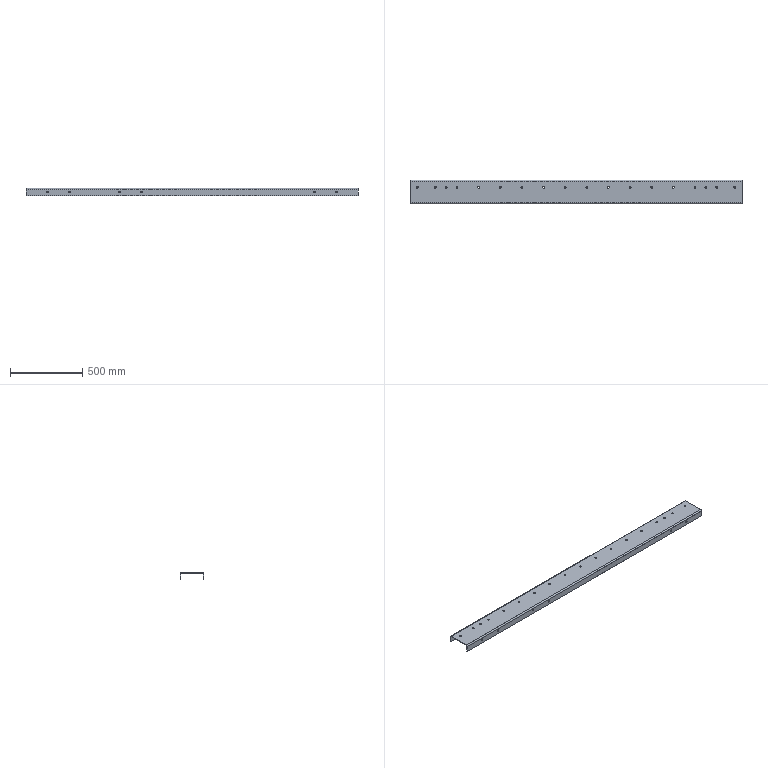Part | STEP file | DCV-000-031-2291L | 1 solid | 86 faces | box 2300 x 165 x 50 mm | volume 2571604 mm3 | cylinder 64 | plane 22 | commonest cylinder face diameters 12.5 x32 11 x12 12 x12 13 x4 9 x2 18 x2